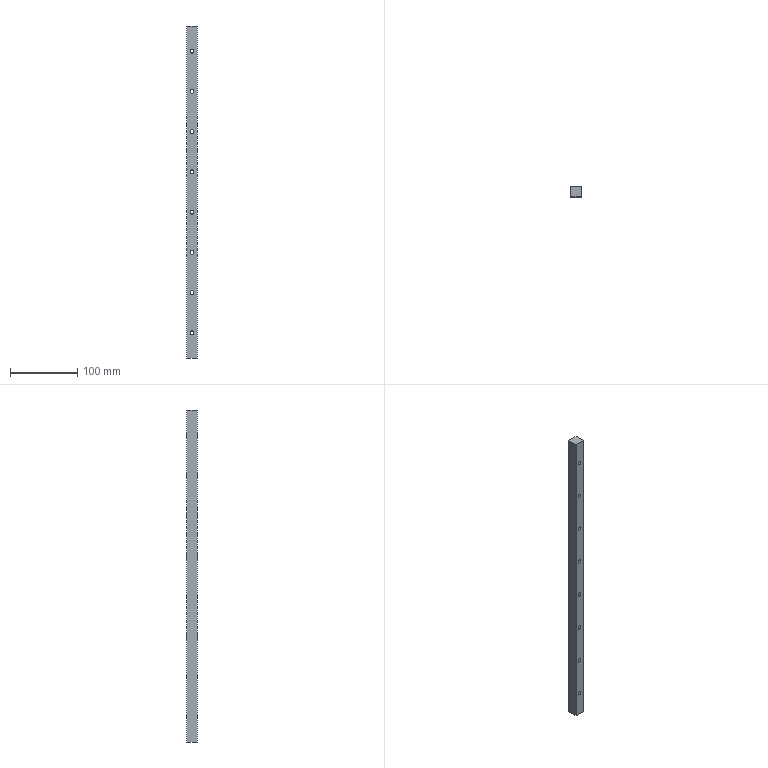Part | 1 solid | 22 faces | box 15 x 15 x 495 mm | volume 107982 mm3 | cylinder 16 | plane 6 | commonest cylinder face diameters 6 x16
STEP:
#1=CARTESIAN_POINT('',(7.5,0.,437.));
#2=VERTEX_POINT('',#1);
#3=CARTESIAN_POINT('',(7.5,0.,443.));
#4=VERTEX_POINT('',#3);
#5=CARTESIAN_POINT('',(7.5,0.,440.));
#6=DIRECTION('',(0.,1.,0.));
#7=DIRECTION('',(0.,0.,1.));
#8=AXIS2_PLACEMENT_3D('',#5,#6,#7);
#9=CIRCLE('',#8,3.);
#10=EDGE_CURVE('',#2,#4,#9,.T.);
#11=ORIENTED_EDGE('',*,*,#10,.F.);
#12=CARTESIAN_POINT('',(7.5,15.,437.));
#13=VERTEX_POINT('',#12);
#14=CARTESIAN_POINT('',(7.5,-35.,437.));
#15=DIRECTION('',(0.,1.,0.));
#16=VECTOR('',#15,1000.);
#17=LINE('',#14,#16);
#18=EDGE_CURVE('',#2,#13,#17,.T.);
#19=ORIENTED_EDGE('',*,*,#18,.T.);
#20=CARTESIAN_POINT('',(7.5,15.,443.));
#21=VERTEX_POINT('',#20);
#22=CARTESIAN_POINT('',(7.5,15.,440.));
#23=DIRECTION('',(0.,1.,0.));
#24=DIRECTION('',(0.,0.,1.));
#25=AXIS2_PLACEMENT_3D('',#22,#23,#24);
#26=CIRCLE('',#25,3.);
#27=EDGE_CURVE('',#13,#21,#26,.T.);
#28=ORIENTED_EDGE('',*,*,#27,.T.);
#29=CARTESIAN_POINT('',(7.5,-35.,443.));
#30=DIRECTION('',(0.,1.,0.));
#31=VECTOR('',#30,1000.);
#32=LINE('',#29,#31);
#33=EDGE_CURVE('',#4,#21,#32,.T.);
#34=ORIENTED_EDGE('',*,*,#33,.F.);
#35=EDGE_LOOP('',(#11,#19,#28,#34));
#36=FACE_OUTER_BOUND('',#35,.T.);
#37=CARTESIAN_POINT('',(7.5,-35.,440.));
#38=DIRECTION('',(0.,1.,0.));
#39=DIRECTION('',(0.,0.,1.));
#40=AXIS2_PLACEMENT_3D('',#37,#38,#39);
#41=CYLINDRICAL_SURFACE('',#40,3.);
#42=ADVANCED_FACE('',(#36),#41,.F.);
#43=CARTESIAN_POINT('',(7.5,0.,377.));
#44=VERTEX_POINT('',#43);
#45=CARTESIAN_POINT('',(7.5,0.,383.));
#46=VERTEX_POINT('',#45);
#47=CARTESIAN_POINT('',(7.5,0.,380.));
#48=DIRECTION('',(0.,1.,0.));
#49=DIRECTION('',(0.,0.,1.));
#50=AXIS2_PLACEMENT_3D('',#47,#48,#49);
#51=CIRCLE('',#50,3.);
#52=EDGE_CURVE('',#44,#46,#51,.T.);
#53=ORIENTED_EDGE('',*,*,#52,.F.);
#54=CARTESIAN_POINT('',(7.5,15.,377.));
#55=VERTEX_POINT('',#54);
#56=CARTESIAN_POINT('',(7.5,-35.,377.));
#57=DIRECTION('',(0.,1.,0.));
#58=VECTOR('',#57,1000.);
#59=LINE('',#56,#58);
#60=EDGE_CURVE('',#44,#55,#59,.T.);
#61=ORIENTED_EDGE('',*,*,#60,.T.);
#62=CARTESIAN_POINT('',(7.5,15.,383.));
#63=VERTEX_POINT('',#62);
#64=CARTESIAN_POINT('',(7.5,15.,380.));
#65=DIRECTION('',(0.,1.,0.));
#66=DIRECTION('',(0.,0.,1.));
#67=AXIS2_PLACEMENT_3D('',#64,#65,#66);
#68=CIRCLE('',#67,3.);
#69=EDGE_CURVE('',#55,#63,#68,.T.);
#70=ORIENTED_EDGE('',*,*,#69,.T.);
#71=CARTESIAN_POINT('',(7.5,-35.,383.));
#72=DIRECTION('',(0.,1.,0.));
#73=VECTOR('',#72,1000.);
#74=LINE('',#71,#73);
#75=EDGE_CURVE('',#46,#63,#74,.T.);
#76=ORIENTED_EDGE('',*,*,#75,.F.);
#77=EDGE_LOOP('',(#53,#61,#70,#76));
#78=FACE_OUTER_BOUND('',#77,.T.);
#79=CARTESIAN_POINT('',(7.5,-35.,380.));
#80=DIRECTION('',(0.,1.,0.));
#81=DIRECTION('',(0.,0.,1.));
#82=AXIS2_PLACEMENT_3D('',#79,#80,#81);
#83=CYLINDRICAL_SURFACE('',#82,3.);
#84=ADVANCED_FACE('',(#78),#83,.F.);
#85=CARTESIAN_POINT('',(7.5,0.,317.));
#86=VERTEX_POINT('',#85);
#87=CARTESIAN_POINT('',(7.5,0.,323.));
#88=VERTEX_POINT('',#87);
#89=CARTESIAN_POINT('',(7.5,0.,320.));
#90=DIRECTION('',(0.,1.,0.));
#91=DIRECTION('',(0.,0.,1.));
#92=AXIS2_PLACEMENT_3D('',#89,#90,#91);
#93=CIRCLE('',#92,3.);
#94=EDGE_CURVE('',#86,#88,#93,.T.);
#95=ORIENTED_EDGE('',*,*,#94,.F.);
#96=CARTESIAN_POINT('',(7.5,15.,317.));
#97=VERTEX_POINT('',#96);
#98=CARTESIAN_POINT('',(7.5,-35.,317.));
#99=DIRECTION('',(0.,1.,0.));
#100=VECTOR('',#99,1000.);
#101=LINE('',#98,#100);
#102=EDGE_CURVE('',#86,#97,#101,.T.);
#103=ORIENTED_EDGE('',*,*,#102,.T.);
#104=CARTESIAN_POINT('',(7.5,15.,323.));
#105=VERTEX_POINT('',#104);
#106=CARTESIAN_POINT('',(7.5,15.,320.));
#107=DIRECTION('',(0.,1.,0.));
#108=DIRECTION('',(0.,0.,1.));
#109=AXIS2_PLACEMENT_3D('',#106,#107,#108);
#110=CIRCLE('',#109,3.);
#111=EDGE_CURVE('',#97,#105,#110,.T.);
#112=ORIENTED_EDGE('',*,*,#111,.T.);
#113=CARTESIAN_POINT('',(7.5,-35.,323.));
#114=DIRECTION('',(0.,1.,0.));
#115=VECTOR('',#114,1000.);
#116=LINE('',#113,#115);
#117=EDGE_CURVE('',#88,#105,#116,.T.);
#118=ORIENTED_EDGE('',*,*,#117,.F.);
#119=EDGE_LOOP('',(#95,#103,#112,#118));
#120=FACE_OUTER_BOUND('',#119,.T.);
#121=CARTESIAN_POINT('',(7.5,-35.,320.));
#122=DIRECTION('',(0.,1.,0.));
#123=DIRECTION('',(0.,0.,1.));
#124=AXIS2_PLACEMENT_3D('',#121,#122,#123);
#125=CYLINDRICAL_SURFACE('',#124,3.);
#126=ADVANCED_FACE('',(#120),#125,.F.);
#127=CARTESIAN_POINT('',(7.5,0.,257.));
#128=VERTEX_POINT('',#127);
#129=CARTESIAN_POINT('',(7.5,0.,263.));
#130=VERTEX_POINT('',#129);
#131=CARTESIAN_POINT('',(7.5,0.,260.));
#132=DIRECTION('',(0.,1.,0.));
#133=DIRECTION('',(0.,0.,1.));
#134=AXIS2_PLACEMENT_3D('',#131,#132,#133);
#135=CIRCLE('',#134,3.);
#136=EDGE_CURVE('',#128,#130,#135,.T.);
#137=ORIENTED_EDGE('',*,*,#136,.F.);
#138=CARTESIAN_POINT('',(7.5,15.,257.));
#139=VERTEX_POINT('',#138);
#140=CARTESIAN_POINT('',(7.5,-35.,257.));
#141=DIRECTION('',(0.,1.,0.));
#142=VECTOR('',#141,1000.);
#143=LINE('',#140,#142);
#144=EDGE_CURVE('',#128,#139,#143,.T.);
#145=ORIENTED_EDGE('',*,*,#144,.T.);
#146=CARTESIAN_POINT('',(7.5,15.,263.));
#147=VERTEX_POINT('',#146);
#148=CARTESIAN_POINT('',(7.5,15.,260.));
#149=DIRECTION('',(0.,1.,0.));
#150=DIRECTION('',(0.,0.,1.));
#151=AXIS2_PLACEMENT_3D('',#148,#149,#150);
#152=CIRCLE('',#151,3.);
#153=EDGE_CURVE('',#139,#147,#152,.T.);
#154=ORIENTED_EDGE('',*,*,#153,.T.);
#155=CARTESIAN_POINT('',(7.5,-35.,263.));
#156=DIRECTION('',(0.,1.,0.));
#157=VECTOR('',#156,1000.);
#158=LINE('',#155,#157);
#159=EDGE_CURVE('',#130,#147,#158,.T.);
#160=ORIENTED_EDGE('',*,*,#159,.F.);
#161=EDGE_LOOP('',(#137,#145,#154,#160));
#162=FACE_OUTER_BOUND('',#161,.T.);
#163=CARTESIAN_POINT('',(7.5,-35.,260.));
#164=DIRECTION('',(0.,1.,0.));
#165=DIRECTION('',(0.,0.,1.));
#166=AXIS2_PLACEMENT_3D('',#163,#164,#165);
#167=CYLINDRICAL_SURFACE('',#166,3.);
#168=ADVANCED_FACE('',(#162),#167,.F.);
#169=CARTESIAN_POINT('',(7.5,0.,197.));
#170=VERTEX_POINT('',#169);
#171=CARTESIAN_POINT('',(7.5,0.,203.));
#172=VERTEX_POINT('',#171);
#173=CARTESIAN_POINT('',(7.5,0.,200.));
#174=DIRECTION('',(0.,1.,0.));
#175=DIRECTION('',(0.,0.,1.));
#176=AXIS2_PLACEMENT_3D('',#173,#174,#175);
#177=CIRCLE('',#176,3.);
#178=EDGE_CURVE('',#170,#172,#177,.T.);
#179=ORIENTED_EDGE('',*,*,#178,.F.);
#180=CARTESIAN_POINT('',(7.5,15.,197.));
#181=VERTEX_POINT('',#180);
#182=CARTESIAN_POINT('',(7.5,-35.,197.));
#183=DIRECTION('',(0.,1.,0.));
#184=VECTOR('',#183,1000.);
#185=LINE('',#182,#184);
#186=EDGE_CURVE('',#170,#181,#185,.T.);
#187=ORIENTED_EDGE('',*,*,#186,.T.);
#188=CARTESIAN_POINT('',(7.5,15.,203.));
#189=VERTEX_POINT('',#188);
#190=CARTESIAN_POINT('',(7.5,15.,200.));
#191=DIRECTION('',(0.,1.,0.));
#192=DIRECTION('',(0.,0.,1.));
#193=AXIS2_PLACEMENT_3D('',#190,#191,#192);
#194=CIRCLE('',#193,3.);
#195=EDGE_CURVE('',#181,#189,#194,.T.);
#196=ORIENTED_EDGE('',*,*,#195,.T.);
#197=CARTESIAN_POINT('',(7.5,-35.,203.));
#198=DIRECTION('',(0.,1.,0.));
#199=VECTOR('',#198,1000.);
#200=LINE('',#197,#199);
#201=EDGE_CURVE('',#172,#189,#200,.T.);
#202=ORIENTED_EDGE('',*,*,#201,.F.);
#203=EDGE_LOOP('',(#179,#187,#196,#202));
#204=FACE_OUTER_BOUND('',#203,.T.);
#205=CARTESIAN_POINT('',(7.5,-35.,200.));
#206=DIRECTION('',(0.,1.,0.));
#207=DIRECTION('',(0.,0.,1.));
#208=AXIS2_PLACEMENT_3D('',#205,#206,#207);
#209=CYLINDRICAL_SURFACE('',#208,3.);
#210=ADVANCED_FACE('',(#204),#209,.F.);
#211=CARTESIAN_POINT('',(7.5,0.,137.));
#212=VERTEX_POINT('',#211);
#213=CARTESIAN_POINT('',(7.5,0.,143.));
#214=VERTEX_POINT('',#213);
#215=CARTESIAN_POINT('',(7.5,0.,140.));
#216=DIRECTION('',(0.,1.,0.));
#217=DIRECTION('',(0.,0.,1.));
#218=AXIS2_PLACEMENT_3D('',#215,#216,#217);
#219=CIRCLE('',#218,3.);
#220=EDGE_CURVE('',#212,#214,#219,.T.);
#221=ORIENTED_EDGE('',*,*,#220,.F.);
#222=CARTESIAN_POINT('',(7.5,15.,137.));
#223=VERTEX_POINT('',#222);
#224=CARTESIAN_POINT('',(7.5,-35.,137.));
#225=DIRECTION('',(0.,1.,0.));
#226=VECTOR('',#225,1000.);
#227=LINE('',#224,#226);
#228=EDGE_CURVE('',#212,#223,#227,.T.);
#229=ORIENTED_EDGE('',*,*,#228,.T.);
#230=CARTESIAN_POINT('',(7.5,15.,143.));
#231=VERTEX_POINT('',#230);
#232=CARTESIAN_POINT('',(7.5,15.,140.));
#233=DIRECTION('',(0.,1.,0.));
#234=DIRECTION('',(0.,0.,1.));
#235=AXIS2_PLACEMENT_3D('',#232,#233,#234);
#236=CIRCLE('',#235,3.);
#237=EDGE_CURVE('',#223,#231,#236,.T.);
#238=ORIENTED_EDGE('',*,*,#237,.T.);
#239=CARTESIAN_POINT('',(7.5,-35.,143.));
#240=DIRECTION('',(0.,1.,0.));
#241=VECTOR('',#240,1000.);
#242=LINE('',#239,#241);
#243=EDGE_CURVE('',#214,#231,#242,.T.);
#244=ORIENTED_EDGE('',*,*,#243,.F.);
#245=EDGE_LOOP('',(#221,#229,#238,#244));
#246=FACE_OUTER_BOUND('',#245,.T.);
#247=CARTESIAN_POINT('',(7.5,-35.,140.));
#248=DIRECTION('',(0.,1.,0.));
#249=DIRECTION('',(0.,0.,1.));
#250=AXIS2_PLACEMENT_3D('',#247,#248,#249);
#251=CYLINDRICAL_SURFACE('',#250,3.);
#252=ADVANCED_FACE('',(#246),#251,.F.);
#253=CARTESIAN_POINT('',(7.5,0.,77.));
#254=VERTEX_POINT('',#253);
#255=CARTESIAN_POINT('',(7.5,0.,83.));
#256=VERTEX_POINT('',#255);
#257=CARTESIAN_POINT('',(7.5,0.,80.));
#258=DIRECTION('',(0.,1.,0.));
#259=DIRECTION('',(0.,0.,1.));
#260=AXIS2_PLACEMENT_3D('',#257,#258,#259);
#261=CIRCLE('',#260,3.);
#262=EDGE_CURVE('',#254,#256,#261,.T.);
#263=ORIENTED_EDGE('',*,*,#262,.F.);
#264=CARTESIAN_POINT('',(7.5,15.,77.));
#265=VERTEX_POINT('',#264);
#266=CARTESIAN_POINT('',(7.5,-35.,77.));
#267=DIRECTION('',(0.,1.,0.));
#268=VECTOR('',#267,1000.);
#269=LINE('',#266,#268);
#270=EDGE_CURVE('',#254,#265,#269,.T.);
#271=ORIENTED_EDGE('',*,*,#270,.T.);
#272=CARTESIAN_POINT('',(7.5,15.,83.));
#273=VERTEX_POINT('',#272);
#274=CARTESIAN_POINT('',(7.5,15.,80.));
#275=DIRECTION('',(0.,1.,0.));
#276=DIRECTION('',(0.,0.,1.));
#277=AXIS2_PLACEMENT_3D('',#274,#275,#276);
#278=CIRCLE('',#277,3.);
#279=EDGE_CURVE('',#265,#273,#278,.T.);
#280=ORIENTED_EDGE('',*,*,#279,.T.);
#281=CARTESIAN_POINT('',(7.5,-35.,83.));
#282=DIRECTION('',(0.,1.,0.));
#283=VECTOR('',#282,1000.);
#284=LINE('',#281,#283);
#285=EDGE_CURVE('',#256,#273,#284,.T.);
#286=ORIENTED_EDGE('',*,*,#285,.F.);
#287=EDGE_LOOP('',(#263,#271,#280,#286));
#288=FACE_OUTER_BOUND('',#287,.T.);
#289=CARTESIAN_POINT('',(7.5,-35.,80.));
#290=DIRECTION('',(0.,1.,0.));
#291=DIRECTION('',(0.,0.,1.));
#292=AXIS2_PLACEMENT_3D('',#289,#290,#291);
#293=CYLINDRICAL_SURFACE('',#292,3.);
#294=ADVANCED_FACE('',(#288),#293,.F.);
#295=CARTESIAN_POINT('',(7.5,0.,17.));
#296=VERTEX_POINT('',#295);
#297=CARTESIAN_POINT('',(7.5,0.,23.));
#298=VERTEX_POINT('',#297);
#299=CARTESIAN_POINT('',(7.5,0.,20.));
#300=DIRECTION('',(0.,1.,0.));
#301=DIRECTION('',(0.,0.,1.));
#302=AXIS2_PLACEMENT_3D('',#299,#300,#301);
#303=CIRCLE('',#302,3.);
#304=EDGE_CURVE('',#296,#298,#303,.T.);
#305=ORIENTED_EDGE('',*,*,#304,.F.);
#306=CARTESIAN_POINT('',(7.5,15.,17.));
#307=VERTEX_POINT('',#306);
#308=CARTESIAN_POINT('',(7.5,-35.,17.));
#309=DIRECTION('',(0.,1.,0.));
#310=VECTOR('',#309,1000.);
#311=LINE('',#308,#310);
#312=EDGE_CURVE('',#296,#307,#311,.T.);
#313=ORIENTED_EDGE('',*,*,#312,.T.);
#314=CARTESIAN_POINT('',(7.5,15.,23.));
#315=VERTEX_POINT('',#314);
#316=CARTESIAN_POINT('',(7.5,15.,20.));
#317=DIRECTION('',(0.,1.,0.));
#318=DIRECTION('',(0.,0.,1.));
#319=AXIS2_PLACEMENT_3D('',#316,#317,#318);
#320=CIRCLE('',#319,3.);
#321=EDGE_CURVE('',#307,#315,#320,.T.);
#322=ORIENTED_EDGE('',*,*,#321,.T.);
#323=CARTESIAN_POINT('',(7.5,-35.,23.));
#324=DIRECTION('',(0.,1.,0.));
#325=VECTOR('',#324,1000.);
#326=LINE('',#323,#325);
#327=EDGE_CURVE('',#298,#315,#326,.T.);
#328=ORIENTED_EDGE('',*,*,#327,.F.);
#329=EDGE_LOOP('',(#305,#313,#322,#328));
#330=FACE_OUTER_BOUND('',#329,.T.);
#331=CARTESIAN_POINT('',(7.5,-35.,20.));
#332=DIRECTION('',(0.,1.,0.));
#333=DIRECTION('',(0.,0.,1.));
#334=AXIS2_PLACEMENT_3D('',#331,#332,#333);
#335=CYLINDRICAL_SURFACE('',#334,3.);
#336=ADVANCED_FACE('',(#330),#335,.F.);
#337=CARTESIAN_POINT('',(0.,15.,477.5));
#338=VERTEX_POINT('',#337);
#339=CARTESIAN_POINT('',(0.,0.,477.5));
#340=VERTEX_POINT('',#339);
#341=CARTESIAN_POINT('',(0.,15.,477.5));
#342=DIRECTION('',(0.,-1.,0.));
#343=VECTOR('',#342,1000.);
#344=LINE('',#341,#343);
#345=EDGE_CURVE('',#338,#340,#344,.T.);
#346=ORIENTED_EDGE('',*,*,#345,.F.);
#347=CARTESIAN_POINT('',(0.,15.,-17.5));
#348=VERTEX_POINT('',#347);
#349=CARTESIAN_POINT('',(0.,15.,495.));
#350=DIRECTION('',(0.,0.,-1.));
#351=VECTOR('',#350,1000.);
#352=LINE('',#349,#351);
#353=EDGE_CURVE('',#338,#348,#352,.T.);
#354=ORIENTED_EDGE('',*,*,#353,.T.);
#355=CARTESIAN_POINT('',(0.,0.,-17.5));
#356=VERTEX_POINT('',#355);
#357=CARTESIAN_POINT('',(0.,0.,-17.5));
#358=DIRECTION('',(0.,1.,0.));
#359=VECTOR('',#358,1000.);
#360=LINE('',#357,#359);
#361=EDGE_CURVE('',#356,#348,#360,.T.);
#362=ORIENTED_EDGE('',*,*,#361,.F.);
#363=CARTESIAN_POINT('',(0.,0.,495.));
#364=DIRECTION('',(0.,0.,-1.));
#365=VECTOR('',#364,1000.);
#366=LINE('',#363,#365);
#367=EDGE_CURVE('',#340,#356,#366,.T.);
#368=ORIENTED_EDGE('',*,*,#367,.F.);
#369=EDGE_LOOP('',(#346,#354,#362,#368));
#370=FACE_OUTER_BOUND('',#369,.T.);
#371=CARTESIAN_POINT('',(0.,0.,495.));
#372=DIRECTION('',(1.,0.,0.));
#373=DIRECTION('',(0.,0.,-1.));
#374=AXIS2_PLACEMENT_3D('',#371,#372,#373);
#375=PLANE('',#374);
#376=ADVANCED_FACE('',(#370),#375,.F.);
#377=CARTESIAN_POINT('',(7.5,0.,20.));
#378=DIRECTION('',(0.,1.,0.));
#379=DIRECTION('',(0.,0.,1.));
#380=AXIS2_PLACEMENT_3D('',#377,#378,#379);
#381=CIRCLE('',#380,3.);
#382=EDGE_CURVE('',#298,#296,#381,.T.);
#383=ORIENTED_EDGE('',*,*,#382,.T.);
#384=ORIENTED_EDGE('',*,*,#304,.T.);
#385=EDGE_LOOP('',(#383,#384));
#386=FACE_BOUND('',#385,.T.);
#387=CARTESIAN_POINT('',(7.5,0.,80.));
#388=DIRECTION('',(0.,1.,0.));
#389=DIRECTION('',(0.,0.,1.));
#390=AXIS2_PLACEMENT_3D('',#387,#388,#389);
#391=CIRCLE('',#390,3.);
#392=EDGE_CURVE('',#256,#254,#391,.T.);
#393=ORIENTED_EDGE('',*,*,#392,.T.);
#394=ORIENTED_EDGE('',*,*,#262,.T.);
#395=EDGE_LOOP('',(#393,#394));
#396=FACE_BOUND('',#395,.T.);
#397=CARTESIAN_POINT('',(7.5,0.,140.));
#398=DIRECTION('',(0.,1.,0.));
#399=DIRECTION('',(0.,0.,1.));
#400=AXIS2_PLACEMENT_3D('',#397,#398,#399);
#401=CIRCLE('',#400,3.);
#402=EDGE_CURVE('',#214,#212,#401,.T.);
#403=ORIENTED_EDGE('',*,*,#402,.T.);
#404=ORIENTED_EDGE('',*,*,#220,.T.);
#405=EDGE_LOOP('',(#403,#404));
#406=FACE_BOUND('',#405,.T.);
#407=CARTESIAN_POINT('',(7.5,0.,200.));
#408=DIRECTION('',(0.,1.,0.));
#409=DIRECTION('',(0.,0.,1.));
#410=AXIS2_PLACEMENT_3D('',#407,#408,#409);
#411=CIRCLE('',#410,3.);
#412=EDGE_CURVE('',#172,#170,#411,.T.);
#413=ORIENTED_EDGE('',*,*,#412,.T.);
#414=ORIENTED_EDGE('',*,*,#178,.T.);
#415=EDGE_LOOP('',(#413,#414));
#416=FACE_BOUND('',#415,.T.);
#417=CARTESIAN_POINT('',(7.5,0.,260.));
#418=DIRECTION('',(0.,1.,0.));
#419=DIRECTION('',(0.,0.,1.));
#420=AXIS2_PLACEMENT_3D('',#417,#418,#419);
#421=CIRCLE('',#420,3.);
#422=EDGE_CURVE('',#130,#128,#421,.T.);
#423=ORIENTED_EDGE('',*,*,#422,.T.);
#424=ORIENTED_EDGE('',*,*,#136,.T.);
#425=EDGE_LOOP('',(#423,#424));
#426=FACE_BOUND('',#425,.T.);
#427=CARTESIAN_POINT('',(7.5,0.,320.));
#428=DIRECTION('',(0.,1.,0.));
#429=DIRECTION('',(0.,0.,1.));
#430=AXIS2_PLACEMENT_3D('',#427,#428,#429);
#431=CIRCLE('',#430,3.);
#432=EDGE_CURVE('',#88,#86,#431,.T.);
#433=ORIENTED_EDGE('',*,*,#432,.T.);
#434=ORIENTED_EDGE('',*,*,#94,.T.);
#435=EDGE_LOOP('',(#433,#434));
#436=FACE_BOUND('',#435,.T.);
#437=CARTESIAN_POINT('',(7.5,0.,380.));
#438=DIRECTION('',(0.,1.,0.));
#439=DIRECTION('',(0.,0.,1.));
#440=AXIS2_PLACEMENT_3D('',#437,#438,#439);
#441=CIRCLE('',#440,3.);
#442=EDGE_CURVE('',#46,#44,#441,.T.);
#443=ORIENTED_EDGE('',*,*,#442,.T.);
#444=ORIENTED_EDGE('',*,*,#52,.T.);
#445=EDGE_LOOP('',(#443,#444));
#446=FACE_BOUND('',#445,.T.);
#447=CARTESIAN_POINT('',(7.5,0.,440.));
#448=DIRECTION('',(0.,1.,0.));
#449=DIRECTION('',(0.,0.,1.));
#450=AXIS2_PLACEMENT_3D('',#447,#448,#449);
#451=CIRCLE('',#450,3.);
#452=EDGE_CURVE('',#4,#2,#451,.T.);
#453=ORIENTED_EDGE('',*,*,#452,.T.);
#454=ORIENTED_EDGE('',*,*,#10,.T.);
#455=EDGE_LOOP('',(#453,#454));
#456=FACE_BOUND('',#455,.T.);
#457=CARTESIAN_POINT('',(15.,0.,477.5));
#458=VERTEX_POINT('',#457);
#459=CARTESIAN_POINT('',(0.,0.,477.5));
#460=DIRECTION('',(1.,0.,0.));
#461=VECTOR('',#460,1000.);
#462=LINE('',#459,#461);
#463=EDGE_CURVE('',#340,#458,#462,.T.);
#464=ORIENTED_EDGE('',*,*,#463,.F.);
#465=ORIENTED_EDGE('',*,*,#367,.T.);
#466=CARTESIAN_POINT('',(15.,0.,-17.5));
#467=VERTEX_POINT('',#466);
#468=CARTESIAN_POINT('',(15.,0.,-17.5));
#469=DIRECTION('',(-1.,0.,0.));
#470=VECTOR('',#469,1000.);
#471=LINE('',#468,#470);
#472=EDGE_CURVE('',#467,#356,#471,.T.);
#473=ORIENTED_EDGE('',*,*,#472,.F.);
#474=CARTESIAN_POINT('',(15.,0.,495.));
#475=DIRECTION('',(0.,0.,-1.));
#476=VECTOR('',#475,1000.);
#477=LINE('',#474,#476);
#478=EDGE_CURVE('',#458,#467,#477,.T.);
#479=ORIENTED_EDGE('',*,*,#478,.F.);
#480=EDGE_LOOP('',(#464,#465,#473,#479));
#481=FACE_OUTER_BOUND('',#480,.T.);
#482=CARTESIAN_POINT('',(0.,0.,495.));
#483=DIRECTION('',(0.,1.,0.));
#484=DIRECTION('',(0.,0.,1.));
#485=AXIS2_PLACEMENT_3D('',#482,#483,#484);
#486=PLANE('',#485);
#487=ADVANCED_FACE('',(#386,#396,#406,#416,#426,#436,#446,#456,#481),#486,.F.);
#488=CARTESIAN_POINT('',(15.,15.,477.5));
#489=VERTEX_POINT('',#488);
#490=CARTESIAN_POINT('',(15.,0.,477.5));
#491=DIRECTION('',(0.,1.,0.));
#492=VECTOR('',#491,1000.);
#493=LINE('',#490,#492);
#494=EDGE_CURVE('',#458,#489,#493,.T.);
#495=ORIENTED_EDGE('',*,*,#494,.F.);
#496=ORIENTED_EDGE('',*,*,#478,.T.);
#497=CARTESIAN_POINT('',(15.,15.,-17.5));
#498=VERTEX_POINT('',#497);
#499=CARTESIAN_POINT('',(15.,15.,-17.5));
#500=DIRECTION('',(0.,-1.,0.));
#501=VECTOR('',#500,1000.);
#502=LINE('',#499,#501);
#503=EDGE_CURVE('',#498,#467,#502,.T.);
#504=ORIENTED_EDGE('',*,*,#503,.F.);
#505=CARTESIAN_POINT('',(15.,15.,495.));
#506=DIRECTION('',(0.,0.,-1.));
#507=VECTOR('',#506,1000.);
#508=LINE('',#505,#507);
#509=EDGE_CURVE('',#489,#498,#508,.T.);
#510=ORIENTED_EDGE('',*,*,#509,.F.);
#511=EDGE_LOOP('',(#495,#496,#504,#510));
#512=FACE_OUTER_BOUND('',#511,.T.);
#513=CARTESIAN_POINT('',(15.,0.,495.));
#514=DIRECTION('',(-1.,0.,0.));
#515=DIRECTION('',(0.,0.,1.));
#516=AXIS2_PLACEMENT_3D('',#513,#514,#515);
#517=PLANE('',#516);
#518=ADVANCED_FACE('',(#512),#517,.F.);
#519=CARTESIAN_POINT('',(7.5,15.,20.));
#520=DIRECTION('',(0.,1.,0.));
#521=DIRECTION('',(0.,0.,1.));
#522=AXIS2_PLACEMENT_3D('',#519,#520,#521);
#523=CIRCLE('',#522,3.);
#524=EDGE_CURVE('',#315,#307,#523,.T.);
#525=ORIENTED_EDGE('',*,*,#524,.F.);
#526=ORIENTED_EDGE('',*,*,#321,.F.);
#527=EDGE_LOOP('',(#525,#526));
#528=FACE_BOUND('',#527,.T.);
#529=CARTESIAN_POINT('',(7.5,15.,80.));
#530=DIRECTION('',(0.,1.,0.));
#531=DIRECTION('',(0.,0.,1.));
#532=AXIS2_PLACEMENT_3D('',#529,#530,#531);
#533=CIRCLE('',#532,3.);
#534=EDGE_CURVE('',#273,#265,#533,.T.);
#535=ORIENTED_EDGE('',*,*,#534,.F.);
#536=ORIENTED_EDGE('',*,*,#279,.F.);
#537=EDGE_LOOP('',(#535,#536));
#538=FACE_BOUND('',#537,.T.);
#539=CARTESIAN_POINT('',(7.5,15.,140.));
#540=DIRECTION('',(0.,1.,0.));
#541=DIRECTION('',(0.,0.,1.));
#542=AXIS2_PLACEMENT_3D('',#539,#540,#541);
#543=CIRCLE('',#542,3.);
#544=EDGE_CURVE('',#231,#223,#543,.T.);
#545=ORIENTED_EDGE('',*,*,#544,.F.);
#546=ORIENTED_EDGE('',*,*,#237,.F.);
#547=EDGE_LOOP('',(#545,#546));
#548=FACE_BOUND('',#547,.T.);
#549=CARTESIAN_POINT('',(7.5,15.,200.));
#550=DIRECTION('',(0.,1.,0.));
#551=DIRECTION('',(0.,0.,1.));
#552=AXIS2_PLACEMENT_3D('',#549,#550,#551);
#553=CIRCLE('',#552,3.);
#554=EDGE_CURVE('',#189,#181,#553,.T.);
#555=ORIENTED_EDGE('',*,*,#554,.F.);
#556=ORIENTED_EDGE('',*,*,#195,.F.);
#557=EDGE_LOOP('',(#555,#556));
#558=FACE_BOUND('',#557,.T.);
#559=CARTESIAN_POINT('',(7.5,15.,260.));
#560=DIRECTION('',(0.,1.,0.));
#561=DIRECTION('',(0.,0.,1.));
#562=AXIS2_PLACEMENT_3D('',#559,#560,#561);
#563=CIRCLE('',#562,3.);
#564=EDGE_CURVE('',#147,#139,#563,.T.);
#565=ORIENTED_EDGE('',*,*,#564,.F.);
#566=ORIENTED_EDGE('',*,*,#153,.F.);
#567=EDGE_LOOP('',(#565,#566));
#568=FACE_BOUND('',#567,.T.);
#569=CARTESIAN_POINT('',(7.5,15.,320.));
#570=DIRECTION('',(0.,1.,0.));
#571=DIRECTION('',(0.,0.,1.));
#572=AXIS2_PLACEMENT_3D('',#569,#570,#571);
#573=CIRCLE('',#572,3.);
#574=EDGE_CURVE('',#105,#97,#573,.T.);
#575=ORIENTED_EDGE('',*,*,#574,.F.);
#576=ORIENTED_EDGE('',*,*,#111,.F.);
#577=EDGE_LOOP('',(#575,#576));
#578=FACE_BOUND('',#577,.T.);
#579=CARTESIAN_POINT('',(7.5,15.,380.));
#580=DIRECTION('',(0.,1.,0.));
#581=DIRECTION('',(0.,0.,1.));
#582=AXIS2_PLACEMENT_3D('',#579,#580,#581);
#583=CIRCLE('',#582,3.);
#584=EDGE_CURVE('',#63,#55,#583,.T.);
#585=ORIENTED_EDGE('',*,*,#584,.F.);
#586=ORIENTED_EDGE('',*,*,#69,.F.);
#587=EDGE_LOOP('',(#585,#586));
#588=FACE_BOUND('',#587,.T.);
#589=CARTESIAN_POINT('',(7.5,15.,440.));
#590=DIRECTION('',(0.,1.,0.));
#591=DIRECTION('',(0.,0.,1.));
#592=AXIS2_PLACEMENT_3D('',#589,#590,#591);
#593=CIRCLE('',#592,3.);
#594=EDGE_CURVE('',#21,#13,#593,.T.);
#595=ORIENTED_EDGE('',*,*,#594,.F.);
#596=ORIENTED_EDGE('',*,*,#27,.F.);
#597=EDGE_LOOP('',(#595,#596));
#598=FACE_BOUND('',#597,.T.);
#599=CARTESIAN_POINT('',(15.,15.,477.5));
#600=DIRECTION('',(-1.,0.,0.));
#601=VECTOR('',#600,1000.);
#602=LINE('',#599,#601);
#603=EDGE_CURVE('',#489,#338,#602,.T.);
#604=ORIENTED_EDGE('',*,*,#603,.F.);
#605=ORIENTED_EDGE('',*,*,#509,.T.);
#606=CARTESIAN_POINT('',(0.,15.,-17.5));
#607=DIRECTION('',(1.,0.,0.));
#608=VECTOR('',#607,1000.);
#609=LINE('',#606,#608);
#610=EDGE_CURVE('',#348,#498,#609,.T.);
#611=ORIENTED_EDGE('',*,*,#610,.F.);
#612=ORIENTED_EDGE('',*,*,#353,.F.);
#613=EDGE_LOOP('',(#604,#605,#611,#612));
#614=FACE_OUTER_BOUND('',#613,.T.);
#615=CARTESIAN_POINT('',(0.,15.,495.));
#616=DIRECTION('',(0.,-1.,0.));
#617=DIRECTION('',(0.,0.,-1.));
#618=AXIS2_PLACEMENT_3D('',#615,#616,#617);
#619=PLANE('',#618);
#620=ADVANCED_FACE('',(#528,#538,#548,#558,#568,#578,#588,#598,#614),#619,.F.);
#621=ORIENTED_EDGE('',*,*,#312,.F.);
#622=ORIENTED_EDGE('',*,*,#382,.F.);
#623=ORIENTED_EDGE('',*,*,#327,.T.);
#624=ORIENTED_EDGE('',*,*,#524,.T.);
#625=EDGE_LOOP('',(#621,#622,#623,#624));
#626=FACE_OUTER_BOUND('',#625,.T.);
#627=CARTESIAN_POINT('',(7.5,-35.,20.));
#628=DIRECTION('',(0.,1.,0.));
#629=DIRECTION('',(0.,0.,1.));
#630=AXIS2_PLACEMENT_3D('',#627,#628,#629);
#631=CYLINDRICAL_SURFACE('',#630,3.);
#632=ADVANCED_FACE('',(#626),#631,.F.);
#633=ORIENTED_EDGE('',*,*,#270,.F.);
#634=ORIENTED_EDGE('',*,*,#392,.F.);
#635=ORIENTED_EDGE('',*,*,#285,.T.);
#636=ORIENTED_EDGE('',*,*,#534,.T.);
#637=EDGE_LOOP('',(#633,#634,#635,#636));
#638=FACE_OUTER_BOUND('',#637,.T.);
#639=CARTESIAN_POINT('',(7.5,-35.,80.));
#640=DIRECTION('',(0.,1.,0.));
#641=DIRECTION('',(0.,0.,1.));
#642=AXIS2_PLACEMENT_3D('',#639,#640,#641);
#643=CYLINDRICAL_SURFACE('',#642,3.);
#644=ADVANCED_FACE('',(#638),#643,.F.);
#645=ORIENTED_EDGE('',*,*,#228,.F.);
#646=ORIENTED_EDGE('',*,*,#402,.F.);
#647=ORIENTED_EDGE('',*,*,#243,.T.);
#648=ORIENTED_EDGE('',*,*,#544,.T.);
#649=EDGE_LOOP('',(#645,#646,#647,#648));
#650=FACE_OUTER_BOUND('',#649,.T.);
#651=CARTESIAN_POINT('',(7.5,-35.,140.));
#652=DIRECTION('',(0.,1.,0.));
#653=DIRECTION('',(0.,0.,1.));
#654=AXIS2_PLACEMENT_3D('',#651,#652,#653);
#655=CYLINDRICAL_SURFACE('',#654,3.);
#656=ADVANCED_FACE('',(#650),#655,.F.);
#657=ORIENTED_EDGE('',*,*,#186,.F.);
#658=ORIENTED_EDGE('',*,*,#412,.F.);
#659=ORIENTED_EDGE('',*,*,#201,.T.);
#660=ORIENTED_EDGE('',*,*,#554,.T.);
#661=EDGE_LOOP('',(#657,#658,#659,#660));
#662=FACE_OUTER_BOUND('',#661,.T.);
#663=CARTESIAN_POINT('',(7.5,-35.,200.));
#664=DIRECTION('',(0.,1.,0.));
#665=DIRECTION('',(0.,0.,1.));
#666=AXIS2_PLACEMENT_3D('',#663,#664,#665);
#667=CYLINDRICAL_SURFACE('',#666,3.);
#668=ADVANCED_FACE('',(#662),#667,.F.);
#669=ORIENTED_EDGE('',*,*,#144,.F.);
#670=ORIENTED_EDGE('',*,*,#422,.F.);
#671=ORIENTED_EDGE('',*,*,#159,.T.);
#672=ORIENTED_EDGE('',*,*,#564,.T.);
#673=EDGE_LOOP('',(#669,#670,#671,#672));
#674=FACE_OUTER_BOUND('',#673,.T.);
#675=CARTESIAN_POINT('',(7.5,-35.,260.));
#676=DIRECTION('',(0.,1.,0.));
#677=DIRECTION('',(0.,0.,1.));
#678=AXIS2_PLACEMENT_3D('',#675,#676,#677);
#679=CYLINDRICAL_SURFACE('',#678,3.);
#680=ADVANCED_FACE('',(#674),#679,.F.);
#681=ORIENTED_EDGE('',*,*,#102,.F.);
#682=ORIENTED_EDGE('',*,*,#432,.F.);
#683=ORIENTED_EDGE('',*,*,#117,.T.);
#684=ORIENTED_EDGE('',*,*,#574,.T.);
#685=EDGE_LOOP('',(#681,#682,#683,#684));
#686=FACE_OUTER_BOUND('',#685,.T.);
#687=CARTESIAN_POINT('',(7.5,-35.,320.));
#688=DIRECTION('',(0.,1.,0.));
#689=DIRECTION('',(0.,0.,1.));
#690=AXIS2_PLACEMENT_3D('',#687,#688,#689);
#691=CYLINDRICAL_SURFACE('',#690,3.);
#692=ADVANCED_FACE('',(#686),#691,.F.);
#693=ORIENTED_EDGE('',*,*,#60,.F.);
#694=ORIENTED_EDGE('',*,*,#442,.F.);
#695=ORIENTED_EDGE('',*,*,#75,.T.);
#696=ORIENTED_EDGE('',*,*,#584,.T.);
#697=EDGE_LOOP('',(#693,#694,#695,#696));
#698=FACE_OUTER_BOUND('',#697,.T.);
#699=CARTESIAN_POINT('',(7.5,-35.,380.));
#700=DIRECTION('',(0.,1.,0.));
#701=DIRECTION('',(0.,0.,1.));
#702=AXIS2_PLACEMENT_3D('',#699,#700,#701);
#703=CYLINDRICAL_SURFACE('',#702,3.);
#704=ADVANCED_FACE('',(#698),#703,.F.);
#705=ORIENTED_EDGE('',*,*,#18,.F.);
#706=ORIENTED_EDGE('',*,*,#452,.F.);
#707=ORIENTED_EDGE('',*,*,#33,.T.);
#708=ORIENTED_EDGE('',*,*,#594,.T.);
#709=EDGE_LOOP('',(#705,#706,#707,#708));
#710=FACE_OUTER_BOUND('',#709,.T.);
#711=CARTESIAN_POINT('',(7.5,-35.,440.));
#712=DIRECTION('',(0.,1.,0.));
#713=DIRECTION('',(0.,0.,1.));
#714=AXIS2_PLACEMENT_3D('',#711,#712,#713);
#715=CYLINDRICAL_SURFACE('',#714,3.);
#716=ADVANCED_FACE('',(#710),#715,.F.);
#717=ORIENTED_EDGE('',*,*,#472,.T.);
#718=ORIENTED_EDGE('',*,*,#361,.T.);
#719=ORIENTED_EDGE('',*,*,#610,.T.);
#720=ORIENTED_EDGE('',*,*,#503,.T.);
#721=EDGE_LOOP('',(#717,#718,#719,#720));
#722=FACE_OUTER_BOUND('',#721,.T.);
#723=CARTESIAN_POINT('',(0.,0.,-17.5));
#724=DIRECTION('',(0.,0.,-1.));
#725=DIRECTION('',(-1.,0.,0.));
#726=AXIS2_PLACEMENT_3D('',#723,#724,#725);
#727=PLANE('',#726);
#728=ADVANCED_FACE('',(#722),#727,.T.);
#729=ORIENTED_EDGE('',*,*,#603,.T.);
#730=ORIENTED_EDGE('',*,*,#345,.T.);
#731=ORIENTED_EDGE('',*,*,#463,.T.);
#732=ORIENTED_EDGE('',*,*,#494,.T.);
#733=EDGE_LOOP('',(#729,#730,#731,#732));
#734=FACE_OUTER_BOUND('',#733,.T.);
#735=CARTESIAN_POINT('',(0.,0.,477.5));
#736=DIRECTION('',(0.,0.,1.));
#737=DIRECTION('',(1.,0.,0.));
#738=AXIS2_PLACEMENT_3D('',#735,#736,#737);
#739=PLANE('',#738);
#740=ADVANCED_FACE('',(#734),#739,.T.);
#741=CLOSED_SHELL('',(#42,#84,#126,#168,#210,#252,#294,#336,#376,#487,#518,#620,#632,#644,#656,#668,#680,#692,#704,#716,#728,#740));
#742=MANIFOLD_SOLID_BREP('',#741);
#743=CARTESIAN_POINT('',(0.,0.,0.));
#744=DIRECTION('',(0.,0.,1.));
#745=DIRECTION('',(1.,0.,0.));
#746=AXIS2_PLACEMENT_3D('',#743,#744,#745);
#747=(LENGTH_UNIT()NAMED_UNIT(*)SI_UNIT(.MILLI.,.METRE.));
#748=UNCERTAINTY_MEASURE_WITH_UNIT(LENGTH_MEASURE(0.00001),#747,'','');
#749=(NAMED_UNIT(*)PLANE_ANGLE_UNIT()SI_UNIT($,.RADIAN.));
#750=(NAMED_UNIT(*)SI_UNIT($,.STERADIAN.)SOLID_ANGLE_UNIT());
#751=(GEOMETRIC_REPRESENTATION_CONTEXT(3)GLOBAL_UNCERTAINTY_ASSIGNED_CONTEXT((#748))GLOBAL_UNIT_ASSIGNED_CONTEXT((#747,#749,#750))REPRESENTATION_CONTEXT('',''));
#752=ADVANCED_BREP_SHAPE_REPRESENTATION('',(#742,#746),#751);